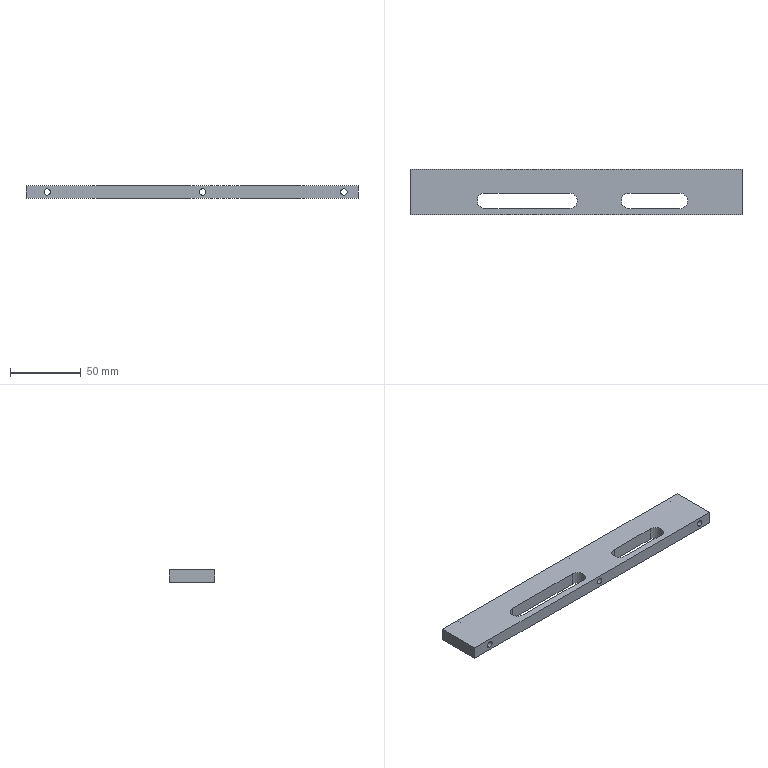Part | STEP file | BU-D02#180a | 1 solid | 31 faces | box 235 x 32.5 x 9 mm | volume 55539 mm3 | cylinder 18 | plane 13 | commonest cylinder face diameters 4.5 x6 8 x6 11 x6